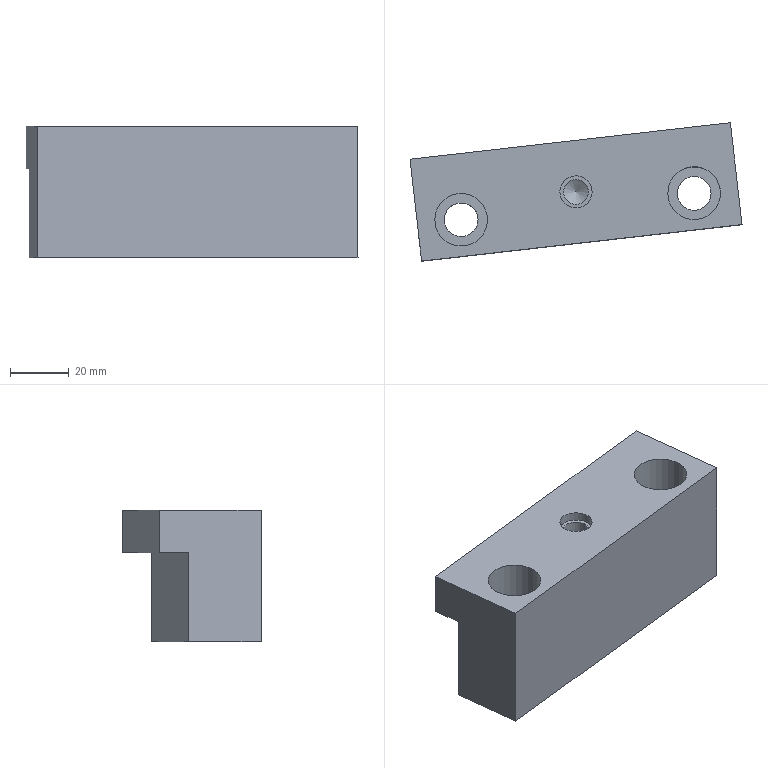Part | NX | features XQ 2 | 1 solid | 18 faces | box 113.255 x 47.227 x 45 mm | volume 123313 mm3 | plane 11 | cylinder 6 | cone 1 | commonest cylinder face diameters 11.5 x2 18 x2 8.5 x1 11 x1
STEP:
#1=CARTESIAN_POINT('',(2664.084,145.075,-123.));
#2=VERTEX_POINT('',#1);
#3=CARTESIAN_POINT('',(2661.254,169.914,-123.));
#4=VERTEX_POINT('',#3);
#5=CARTESIAN_POINT('',(2661.254,169.914,-123.));
#6=DIRECTION('',(-0.1132,0.9936,0.));
#7=VECTOR('',#6,1000.);
#8=LINE('',#5,#7);
#9=EDGE_CURVE('',#2,#4,#8,.T.);
#10=ORIENTED_EDGE('',*,*,#9,.T.);
#11=CARTESIAN_POINT('',(2770.546,182.367,-123.));
#12=VERTEX_POINT('',#11);
#13=CARTESIAN_POINT('',(1119.037,-5.799,-123.));
#14=DIRECTION('',(0.9936,0.1132,0.000000001));
#15=VECTOR('',#14,1000.);
#16=LINE('',#13,#15);
#17=EDGE_CURVE('',#4,#12,#16,.T.);
#18=ORIENTED_EDGE('',*,*,#17,.T.);
#19=CARTESIAN_POINT('',(2773.377,157.527,-123.));
#20=VERTEX_POINT('',#19);
#21=CARTESIAN_POINT('',(2770.546,182.367,-123.));
#22=DIRECTION('',(-0.1132,0.9936,0.));
#23=VECTOR('',#22,1000.);
#24=LINE('',#21,#23);
#25=EDGE_CURVE('',#20,#12,#24,.T.);
#26=ORIENTED_EDGE('',*,*,#25,.F.);
#27=CARTESIAN_POINT('',(1121.867,-30.638,-123.));
#28=DIRECTION('',(0.9936,0.1132,0.000000001));
#29=VECTOR('',#28,1000.);
#30=LINE('',#27,#29);
#31=EDGE_CURVE('',#2,#20,#30,.T.);
#32=ORIENTED_EDGE('',*,*,#31,.F.);
#33=EDGE_LOOP('',(#10,#18,#26,#32));
#34=FACE_BOUND('',#33,.T.);
#35=CARTESIAN_POINT('',(2762.808,168.249,-123.));
#36=VERTEX_POINT('',#35);
#37=CARTESIAN_POINT('',(2757.058,168.249,-123.));
#38=DIRECTION('',(-0.000000001,0.,1.));
#39=DIRECTION('',(1.,0.,0.000000001));
#40=AXIS2_PLACEMENT_3D('',#37,#38,#39);
#41=CIRCLE('',#40,5.75);
#42=EDGE_CURVE('',#36,#36,#41,.T.);
#43=ORIENTED_EDGE('',*,*,#42,.T.);
#44=EDGE_LOOP('',(#43));
#45=FACE_BOUND('',#44,.T.);
#46=CARTESIAN_POINT('',(2683.322,159.193,-123.));
#47=VERTEX_POINT('',#46);
#48=CARTESIAN_POINT('',(2677.572,159.193,-123.));
#49=DIRECTION('',(0.000000001,0.,-1.));
#50=DIRECTION('',(1.,0.,0.000000001));
#51=AXIS2_PLACEMENT_3D('',#48,#49,#50);
#52=CIRCLE('',#51,5.75);
#53=EDGE_CURVE('',#47,#47,#52,.T.);
#54=ORIENTED_EDGE('',*,*,#53,.F.);
#55=EDGE_LOOP('',(#54));
#56=FACE_BOUND('',#55,.T.);
#57=CARTESIAN_POINT('',(1119.037,-5.799,-123.));
#58=DIRECTION('',(-0.000000001,0.,1.));
#59=DIRECTION('',(-0.9936,-0.1132,-0.000000001));
#60=AXIS2_PLACEMENT_3D('',#57,#58,#59);
#61=PLANE('',#60);
#62=ADVANCED_FACE('',(#34,#45,#56),#61,.F.);
#63=CARTESIAN_POINT('',(2722.239,168.353,-78.));
#64=VERTEX_POINT('',#63);
#65=CARTESIAN_POINT('',(2716.749,168.689,-78.));
#66=DIRECTION('',(0.000000001,0.,-1.));
#67=DIRECTION('',(0.9981,-0.06105,0.000000001));
#68=AXIS2_PLACEMENT_3D('',#65,#66,#67);
#69=CIRCLE('',#68,5.5);
#70=EDGE_CURVE('',#64,#64,#69,.T.);
#71=ORIENTED_EDGE('',*,*,#70,.T.);
#72=EDGE_LOOP('',(#71));
#73=FACE_BOUND('',#72,.T.);
#74=CARTESIAN_POINT('',(2660.122,179.85,-78.));
#75=VERTEX_POINT('',#74);
#76=CARTESIAN_POINT('',(2769.414,192.302,-78.));
#77=VERTEX_POINT('',#76);
#78=CARTESIAN_POINT('',(2725.697,187.322,-78.));
#79=DIRECTION('',(0.9936,0.1132,0.000000001));
#80=VECTOR('',#79,1000.);
#81=LINE('',#78,#80);
#82=EDGE_CURVE('',#75,#77,#81,.T.);
#83=ORIENTED_EDGE('',*,*,#82,.F.);
#84=CARTESIAN_POINT('',(2664.084,145.075,-78.));
#85=VERTEX_POINT('',#84);
#86=CARTESIAN_POINT('',(2642.813,331.762,-78.));
#87=DIRECTION('',(-0.1132,0.9936,0.));
#88=VECTOR('',#87,1000.);
#89=LINE('',#86,#88);
#90=EDGE_CURVE('',#85,#75,#89,.T.);
#91=ORIENTED_EDGE('',*,*,#90,.F.);
#92=CARTESIAN_POINT('',(2773.377,157.527,-78.));
#93=VERTEX_POINT('',#92);
#94=CARTESIAN_POINT('',(2750.524,154.924,-78.));
#95=DIRECTION('',(0.9936,0.1132,0.000000001));
#96=VECTOR('',#95,1000.);
#97=LINE('',#94,#96);
#98=EDGE_CURVE('',#85,#93,#97,.T.);
#99=ORIENTED_EDGE('',*,*,#98,.T.);
#100=CARTESIAN_POINT('',(2755.717,312.525,-78.));
#101=DIRECTION('',(-0.1132,0.9936,0.));
#102=VECTOR('',#101,1000.);
#103=LINE('',#100,#102);
#104=EDGE_CURVE('',#93,#77,#103,.T.);
#105=ORIENTED_EDGE('',*,*,#104,.T.);
#106=EDGE_LOOP('',(#83,#91,#99,#105));
#107=FACE_BOUND('',#106,.T.);
#108=CARTESIAN_POINT('',(2766.058,168.249,-78.));
#109=VERTEX_POINT('',#108);
#110=CARTESIAN_POINT('',(2757.058,168.249,-78.));
#111=DIRECTION('',(0.000000001,0.,-1.));
#112=DIRECTION('',(1.,0.,0.000000001));
#113=AXIS2_PLACEMENT_3D('',#110,#111,#112);
#114=CIRCLE('',#113,9.);
#115=EDGE_CURVE('',#109,#109,#114,.T.);
#116=ORIENTED_EDGE('',*,*,#115,.T.);
#117=EDGE_LOOP('',(#116));
#118=FACE_BOUND('',#117,.T.);
#119=CARTESIAN_POINT('',(2686.572,159.193,-78.));
#120=VERTEX_POINT('',#119);
#121=CARTESIAN_POINT('',(2677.572,159.193,-78.));
#122=DIRECTION('',(-0.000000001,0.,1.));
#123=DIRECTION('',(1.,0.,0.000000001));
#124=AXIS2_PLACEMENT_3D('',#121,#122,#123);
#125=CIRCLE('',#124,9.);
#126=EDGE_CURVE('',#120,#120,#125,.T.);
#127=ORIENTED_EDGE('',*,*,#126,.F.);
#128=EDGE_LOOP('',(#127));
#129=FACE_BOUND('',#128,.T.);
#130=CARTESIAN_POINT('',(1973.887,255.547,-78.));
#131=DIRECTION('',(-0.000000001,0.,1.));
#132=DIRECTION('',(0.9981,-0.06105,0.000000001));
#133=AXIS2_PLACEMENT_3D('',#130,#131,#132);
#134=PLANE('',#133);
#135=ADVANCED_FACE('',(#73,#107,#118,#129),#134,.T.);
#136=CARTESIAN_POINT('',(2660.122,179.85,-92.5));
#137=VERTEX_POINT('',#136);
#138=CARTESIAN_POINT('',(2661.254,169.914,-92.5));
#139=VERTEX_POINT('',#138);
#140=CARTESIAN_POINT('',(2661.254,169.914,-92.5));
#141=DIRECTION('',(0.1132,-0.9936,0.));
#142=VECTOR('',#141,1000.);
#143=LINE('',#140,#142);
#144=EDGE_CURVE('',#137,#139,#143,.T.);
#145=ORIENTED_EDGE('',*,*,#144,.T.);
#146=CARTESIAN_POINT('',(2661.254,169.914,-98.027));
#147=DIRECTION('',(0.000000001,0.,-1.));
#148=VECTOR('',#147,1000.);
#149=LINE('',#146,#148);
#150=EDGE_CURVE('',#139,#4,#149,.T.);
#151=ORIENTED_EDGE('',*,*,#150,.T.);
#152=ORIENTED_EDGE('',*,*,#9,.F.);
#153=CARTESIAN_POINT('',(2664.084,145.075,-98.027));
#154=DIRECTION('',(0.000000001,0.,-1.));
#155=VECTOR('',#154,1000.);
#156=LINE('',#153,#155);
#157=EDGE_CURVE('',#85,#2,#156,.T.);
#158=ORIENTED_EDGE('',*,*,#157,.F.);
#159=ORIENTED_EDGE('',*,*,#90,.T.);
#160=CARTESIAN_POINT('',(2660.122,179.85,-98.027));
#161=DIRECTION('',(0.000000001,0.,-1.));
#162=VECTOR('',#161,1000.);
#163=LINE('',#160,#162);
#164=EDGE_CURVE('',#75,#137,#163,.T.);
#165=ORIENTED_EDGE('',*,*,#164,.T.);
#166=EDGE_LOOP('',(#145,#151,#152,#158,#159,#165));
#167=FACE_BOUND('',#166,.T.);
#168=CARTESIAN_POINT('',(2661.254,169.914,-98.027));
#169=DIRECTION('',(0.9936,0.1132,0.000000001));
#170=DIRECTION('',(-0.000000001,0.,1.));
#171=AXIS2_PLACEMENT_3D('',#168,#169,#170);
#172=PLANE('',#171);
#173=ADVANCED_FACE('',(#167),#172,.F.);
#174=CARTESIAN_POINT('',(2769.414,192.302,-92.5));
#175=VERTEX_POINT('',#174);
#176=CARTESIAN_POINT('',(2769.414,192.302,-51.063));
#177=DIRECTION('',(0.000000001,0.,-1.));
#178=VECTOR('',#177,1000.);
#179=LINE('',#176,#178);
#180=EDGE_CURVE('',#77,#175,#179,.T.);
#181=ORIENTED_EDGE('',*,*,#180,.F.);
#182=ORIENTED_EDGE('',*,*,#104,.F.);
#183=CARTESIAN_POINT('',(2773.377,157.527,-58.563));
#184=DIRECTION('',(0.000000001,0.,-1.));
#185=VECTOR('',#184,1000.);
#186=LINE('',#183,#185);
#187=EDGE_CURVE('',#93,#20,#186,.T.);
#188=ORIENTED_EDGE('',*,*,#187,.T.);
#189=ORIENTED_EDGE('',*,*,#25,.T.);
#190=CARTESIAN_POINT('',(2770.546,182.367,-92.5));
#191=VERTEX_POINT('',#190);
#192=CARTESIAN_POINT('',(2770.546,182.367,-58.563));
#193=DIRECTION('',(0.000000001,0.,-1.));
#194=VECTOR('',#193,1000.);
#195=LINE('',#192,#194);
#196=EDGE_CURVE('',#191,#12,#195,.T.);
#197=ORIENTED_EDGE('',*,*,#196,.F.);
#198=CARTESIAN_POINT('',(2755.717,312.525,-92.5));
#199=DIRECTION('',(-0.1132,0.9936,0.));
#200=VECTOR('',#199,1000.);
#201=LINE('',#198,#200);
#202=EDGE_CURVE('',#191,#175,#201,.T.);
#203=ORIENTED_EDGE('',*,*,#202,.T.);
#204=EDGE_LOOP('',(#181,#182,#188,#189,#197,#203));
#205=FACE_BOUND('',#204,.T.);
#206=CARTESIAN_POINT('',(2755.717,312.525,-88.));
#207=DIRECTION('',(-0.9936,-0.1132,-0.000000001));
#208=DIRECTION('',(0.1132,-0.9936,0.));
#209=AXIS2_PLACEMENT_3D('',#206,#207,#208);
#210=PLANE('',#209);
#211=ADVANCED_FACE('',(#205),#210,.F.);
#212=ORIENTED_EDGE('',*,*,#187,.F.);
#213=ORIENTED_EDGE('',*,*,#98,.F.);
#214=ORIENTED_EDGE('',*,*,#157,.T.);
#215=ORIENTED_EDGE('',*,*,#31,.T.);
#216=EDGE_LOOP('',(#212,#213,#214,#215));
#217=FACE_BOUND('',#216,.T.);
#218=CARTESIAN_POINT('',(2750.524,154.924,-58.563));
#219=DIRECTION('',(0.1132,-0.9936,0.));
#220=DIRECTION('',(0.9936,0.1132,0.000000001));
#221=AXIS2_PLACEMENT_3D('',#218,#219,#220);
#222=PLANE('',#221);
#223=ADVANCED_FACE('',(#217),#222,.T.);
#224=ORIENTED_EDGE('',*,*,#150,.F.);
#225=CARTESIAN_POINT('',(2747.694,179.763,-92.5));
#226=DIRECTION('',(0.9936,0.1132,0.000000001));
#227=VECTOR('',#226,1000.);
#228=LINE('',#225,#227);
#229=EDGE_CURVE('',#139,#191,#228,.T.);
#230=ORIENTED_EDGE('',*,*,#229,.T.);
#231=ORIENTED_EDGE('',*,*,#196,.T.);
#232=ORIENTED_EDGE('',*,*,#17,.F.);
#233=EDGE_LOOP('',(#224,#230,#231,#232));
#234=FACE_BOUND('',#233,.T.);
#235=CARTESIAN_POINT('',(2747.694,179.763,-58.563));
#236=DIRECTION('',(0.1132,-0.9936,0.));
#237=DIRECTION('',(0.9936,0.1132,0.000000001));
#238=AXIS2_PLACEMENT_3D('',#235,#236,#237);
#239=PLANE('',#238);
#240=ADVANCED_FACE('',(#234),#239,.F.);
#241=ORIENTED_EDGE('',*,*,#229,.F.);
#242=ORIENTED_EDGE('',*,*,#144,.F.);
#243=CARTESIAN_POINT('',(1991.196,103.636,-92.5));
#244=DIRECTION('',(-0.9936,-0.1132,-0.000000001));
#245=VECTOR('',#244,1000.);
#246=LINE('',#243,#245);
#247=EDGE_CURVE('',#175,#137,#246,.T.);
#248=ORIENTED_EDGE('',*,*,#247,.F.);
#249=ORIENTED_EDGE('',*,*,#202,.F.);
#250=EDGE_LOOP('',(#241,#242,#248,#249));
#251=FACE_BOUND('',#250,.T.);
#252=CARTESIAN_POINT('',(1973.887,255.547,-92.5));
#253=DIRECTION('',(-0.000000001,0.,1.));
#254=DIRECTION('',(0.9981,-0.06105,0.000000001));
#255=AXIS2_PLACEMENT_3D('',#252,#253,#254);
#256=PLANE('',#255);
#257=ADVANCED_FACE('',(#251),#256,.F.);
#258=ORIENTED_EDGE('',*,*,#247,.T.);
#259=ORIENTED_EDGE('',*,*,#164,.F.);
#260=ORIENTED_EDGE('',*,*,#82,.T.);
#261=ORIENTED_EDGE('',*,*,#180,.T.);
#262=EDGE_LOOP('',(#258,#259,#260,#261));
#263=FACE_BOUND('',#262,.T.);
#264=CARTESIAN_POINT('',(2725.697,187.322,-51.063));
#265=DIRECTION('',(0.1132,-0.9936,0.));
#266=DIRECTION('',(0.9936,0.1132,0.000000001));
#267=AXIS2_PLACEMENT_3D('',#264,#265,#266);
#268=PLANE('',#267);
#269=ADVANCED_FACE('',(#263),#268,.F.);
#270=CARTESIAN_POINT('',(2751.308,168.249,-98.));
#271=VERTEX_POINT('',#270);
#272=CARTESIAN_POINT('',(2757.058,168.249,-98.));
#273=DIRECTION('',(0.000000001,0.,-1.));
#274=DIRECTION('',(-1.,0.,-0.000000001));
#275=AXIS2_PLACEMENT_3D('',#272,#273,#274);
#276=CIRCLE('',#275,5.75);
#277=EDGE_CURVE('',#271,#271,#276,.T.);
#278=ORIENTED_EDGE('',*,*,#277,.F.);
#279=EDGE_LOOP('',(#278));
#280=FACE_BOUND('',#279,.T.);
#281=ORIENTED_EDGE('',*,*,#42,.F.);
#282=EDGE_LOOP('',(#281));
#283=FACE_BOUND('',#282,.T.);
#284=CARTESIAN_POINT('',(2757.058,168.249,-73.));
#285=DIRECTION('',(0.000000001,0.,-1.));
#286=DIRECTION('',(-0.9588,-0.284,-0.000000001));
#287=AXIS2_PLACEMENT_3D('',#284,#285,#286);
#288=CYLINDRICAL_SURFACE('',#287,5.75);
#289=ADVANCED_FACE('',(#280,#283),#288,.F.);
#290=ORIENTED_EDGE('',*,*,#277,.T.);
#291=EDGE_LOOP('',(#290));
#292=FACE_BOUND('',#291,.T.);
#293=CARTESIAN_POINT('',(2748.058,168.249,-98.));
#294=VERTEX_POINT('',#293);
#295=CARTESIAN_POINT('',(2757.058,168.249,-98.));
#296=DIRECTION('',(0.000000001,0.,-1.));
#297=DIRECTION('',(-1.,0.,-0.000000001));
#298=AXIS2_PLACEMENT_3D('',#295,#296,#297);
#299=CIRCLE('',#298,9.);
#300=EDGE_CURVE('',#294,#294,#299,.T.);
#301=ORIENTED_EDGE('',*,*,#300,.F.);
#302=EDGE_LOOP('',(#301));
#303=FACE_BOUND('',#302,.T.);
#304=CARTESIAN_POINT('',(2757.058,168.249,-98.));
#305=DIRECTION('',(0.000000001,0.,-1.));
#306=DIRECTION('',(0.9588,0.284,0.000000001));
#307=AXIS2_PLACEMENT_3D('',#304,#305,#306);
#308=PLANE('',#307);
#309=ADVANCED_FACE('',(#292,#303),#308,.F.);
#310=ORIENTED_EDGE('',*,*,#300,.T.);
#311=EDGE_LOOP('',(#310));
#312=FACE_BOUND('',#311,.T.);
#313=ORIENTED_EDGE('',*,*,#115,.F.);
#314=EDGE_LOOP('',(#313));
#315=FACE_BOUND('',#314,.T.);
#316=CARTESIAN_POINT('',(2757.058,168.249,-73.));
#317=DIRECTION('',(0.000000001,0.,-1.));
#318=DIRECTION('',(-0.9588,-0.284,-0.000000001));
#319=AXIS2_PLACEMENT_3D('',#316,#317,#318);
#320=CYLINDRICAL_SURFACE('',#319,9.);
#321=ADVANCED_FACE('',(#312,#315),#320,.F.);
#322=CARTESIAN_POINT('',(2671.822,159.193,-98.));
#323=VERTEX_POINT('',#322);
#324=CARTESIAN_POINT('',(2677.572,159.193,-98.));
#325=DIRECTION('',(-0.000000001,0.,1.));
#326=DIRECTION('',(-1.,0.,-0.000000001));
#327=AXIS2_PLACEMENT_3D('',#324,#325,#326);
#328=CIRCLE('',#327,5.75);
#329=EDGE_CURVE('',#323,#323,#328,.T.);
#330=ORIENTED_EDGE('',*,*,#329,.T.);
#331=EDGE_LOOP('',(#330));
#332=FACE_BOUND('',#331,.T.);
#333=ORIENTED_EDGE('',*,*,#53,.T.);
#334=EDGE_LOOP('',(#333));
#335=FACE_BOUND('',#334,.T.);
#336=CARTESIAN_POINT('',(2677.572,159.193,-73.));
#337=DIRECTION('',(0.000000001,0.,-1.));
#338=DIRECTION('',(0.9981,-0.06105,0.000000001));
#339=AXIS2_PLACEMENT_3D('',#336,#337,#338);
#340=CYLINDRICAL_SURFACE('',#339,5.75);
#341=ADVANCED_FACE('',(#332,#335),#340,.F.);
#342=ORIENTED_EDGE('',*,*,#329,.F.);
#343=EDGE_LOOP('',(#342));
#344=FACE_BOUND('',#343,.T.);
#345=CARTESIAN_POINT('',(2668.572,159.193,-98.));
#346=VERTEX_POINT('',#345);
#347=CARTESIAN_POINT('',(2677.572,159.193,-98.));
#348=DIRECTION('',(-0.000000001,0.,1.));
#349=DIRECTION('',(-1.,0.,-0.000000001));
#350=AXIS2_PLACEMENT_3D('',#347,#348,#349);
#351=CIRCLE('',#350,9.);
#352=EDGE_CURVE('',#346,#346,#351,.T.);
#353=ORIENTED_EDGE('',*,*,#352,.T.);
#354=EDGE_LOOP('',(#353));
#355=FACE_BOUND('',#354,.T.);
#356=CARTESIAN_POINT('',(2677.572,159.193,-98.));
#357=DIRECTION('',(0.000000001,0.,-1.));
#358=DIRECTION('',(-0.9981,0.06105,-0.000000001));
#359=AXIS2_PLACEMENT_3D('',#356,#357,#358);
#360=PLANE('',#359);
#361=ADVANCED_FACE('',(#344,#355),#360,.F.);
#362=ORIENTED_EDGE('',*,*,#352,.F.);
#363=EDGE_LOOP('',(#362));
#364=FACE_BOUND('',#363,.T.);
#365=ORIENTED_EDGE('',*,*,#126,.T.);
#366=EDGE_LOOP('',(#365));
#367=FACE_BOUND('',#366,.T.);
#368=CARTESIAN_POINT('',(2677.572,159.193,-73.));
#369=DIRECTION('',(0.000000001,0.,-1.));
#370=DIRECTION('',(0.9981,-0.06105,0.000000001));
#371=AXIS2_PLACEMENT_3D('',#368,#369,#370);
#372=CYLINDRICAL_SURFACE('',#371,9.);
#373=ADVANCED_FACE('',(#364,#367),#372,.F.);
#374=CARTESIAN_POINT('',(2711.259,169.025,-81.));
#375=VERTEX_POINT('',#374);
#376=CARTESIAN_POINT('',(2716.749,168.689,-81.));
#377=DIRECTION('',(0.000000001,0.,-1.));
#378=DIRECTION('',(-0.9981,0.06105,-0.000000001));
#379=AXIS2_PLACEMENT_3D('',#376,#377,#378);
#380=CIRCLE('',#379,5.5);
#381=EDGE_CURVE('',#375,#375,#380,.T.);
#382=ORIENTED_EDGE('',*,*,#381,.F.);
#383=EDGE_LOOP('',(#382));
#384=FACE_BOUND('',#383,.T.);
#385=CARTESIAN_POINT('',(2712.507,168.948,-81.));
#386=VERTEX_POINT('',#385);
#387=CARTESIAN_POINT('',(2716.749,168.689,-81.));
#388=DIRECTION('',(0.000000001,0.,-1.));
#389=DIRECTION('',(-0.9981,0.06105,-0.000000001));
#390=AXIS2_PLACEMENT_3D('',#387,#388,#389);
#391=CIRCLE('',#390,4.25);
#392=EDGE_CURVE('',#386,#386,#391,.T.);
#393=ORIENTED_EDGE('',*,*,#392,.T.);
#394=EDGE_LOOP('',(#393));
#395=FACE_BOUND('',#394,.T.);
#396=CARTESIAN_POINT('',(2716.749,168.689,-81.));
#397=DIRECTION('',(0.000000001,0.,-1.));
#398=DIRECTION('',(-0.9981,0.06105,-0.000000001));
#399=AXIS2_PLACEMENT_3D('',#396,#397,#398);
#400=PLANE('',#399);
#401=ADVANCED_FACE('',(#384,#395),#400,.F.);
#402=ORIENTED_EDGE('',*,*,#70,.F.);
#403=EDGE_LOOP('',(#402));
#404=FACE_BOUND('',#403,.T.);
#405=ORIENTED_EDGE('',*,*,#381,.T.);
#406=EDGE_LOOP('',(#405));
#407=FACE_BOUND('',#406,.T.);
#408=CARTESIAN_POINT('',(2716.749,168.689,-54.));
#409=DIRECTION('',(0.000000001,0.,-1.));
#410=DIRECTION('',(-0.9981,0.06105,-0.000000001));
#411=AXIS2_PLACEMENT_3D('',#408,#409,#410);
#412=CYLINDRICAL_SURFACE('',#411,5.5);
#413=ADVANCED_FACE('',(#404,#407),#412,.F.);
#414=CARTESIAN_POINT('',(2712.507,168.948,-93.));
#415=VERTEX_POINT('',#414);
#416=CARTESIAN_POINT('',(2716.749,168.689,-93.));
#417=DIRECTION('',(0.000000001,0.,-1.));
#418=DIRECTION('',(-0.9981,0.06105,-0.000000001));
#419=AXIS2_PLACEMENT_3D('',#416,#417,#418);
#420=CIRCLE('',#419,4.25);
#421=EDGE_CURVE('',#415,#415,#420,.T.);
#422=ORIENTED_EDGE('',*,*,#421,.F.);
#423=EDGE_LOOP('',(#422));
#424=FACE_BOUND('',#423,.T.);
#425=CARTESIAN_POINT('',(2716.749,168.689,-95.554));
#426=VERTEX_POINT('',#425);
#427=VERTEX_LOOP('',#426);
#428=FACE_BOUND('',#427,.T.);
#429=CARTESIAN_POINT('',(2716.749,168.689,-93.));
#430=DIRECTION('',(-0.000000001,0.,1.));
#431=DIRECTION('',(0.9981,-0.06105,0.000000001));
#432=AXIS2_PLACEMENT_3D('',#429,#430,#431);
#433=CONICAL_SURFACE('',#432,4.25,1.03);
#434=ADVANCED_FACE('',(#424,#428),#433,.F.);
#435=ORIENTED_EDGE('',*,*,#392,.F.);
#436=EDGE_LOOP('',(#435));
#437=FACE_BOUND('',#436,.T.);
#438=ORIENTED_EDGE('',*,*,#421,.T.);
#439=EDGE_LOOP('',(#438));
#440=FACE_BOUND('',#439,.T.);
#441=CARTESIAN_POINT('',(2716.749,168.689,-73.));
#442=DIRECTION('',(0.000000001,0.,-1.));
#443=DIRECTION('',(-0.9981,0.06105,-0.000000001));
#444=AXIS2_PLACEMENT_3D('',#441,#442,#443);
#445=CYLINDRICAL_SURFACE('',#444,4.25);
#446=ADVANCED_FACE('',(#437,#440),#445,.F.);
#447=CLOSED_SHELL('',(#62,#135,#173,#211,#223,#240,#257,#269,#289,#309,#321,#341,#361,#373,#401,#413,#434,#446));
#448=MANIFOLD_SOLID_BREP('',#447);
#449=(LENGTH_UNIT()NAMED_UNIT(*)SI_UNIT(.MILLI.,.METRE.));
#450=UNCERTAINTY_MEASURE_WITH_UNIT(LENGTH_MEASURE(0.00001),#449,'','');
#451=(NAMED_UNIT(*)PLANE_ANGLE_UNIT()SI_UNIT($,.RADIAN.));
#452=(NAMED_UNIT(*)SI_UNIT($,.STERADIAN.)SOLID_ANGLE_UNIT());
#453=(GEOMETRIC_REPRESENTATION_CONTEXT(3)GLOBAL_UNCERTAINTY_ASSIGNED_CONTEXT((#450))GLOBAL_UNIT_ASSIGNED_CONTEXT((#449,#451,#452))REPRESENTATION_CONTEXT('',''));
#454=ADVANCED_BREP_SHAPE_REPRESENTATION('',(#448),#453);